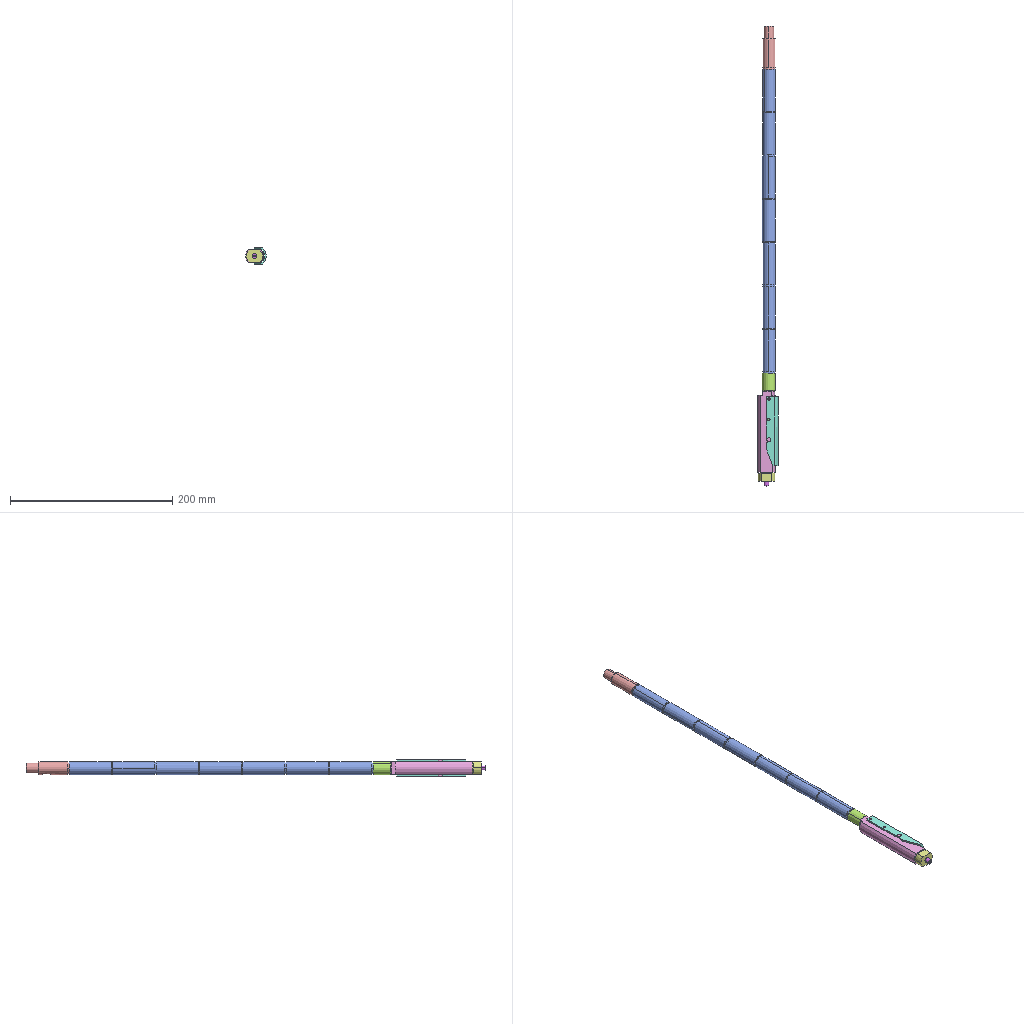Assembly | SolidWorks | 12 different items | 20 placed | box 25 x 567 x 20 mm
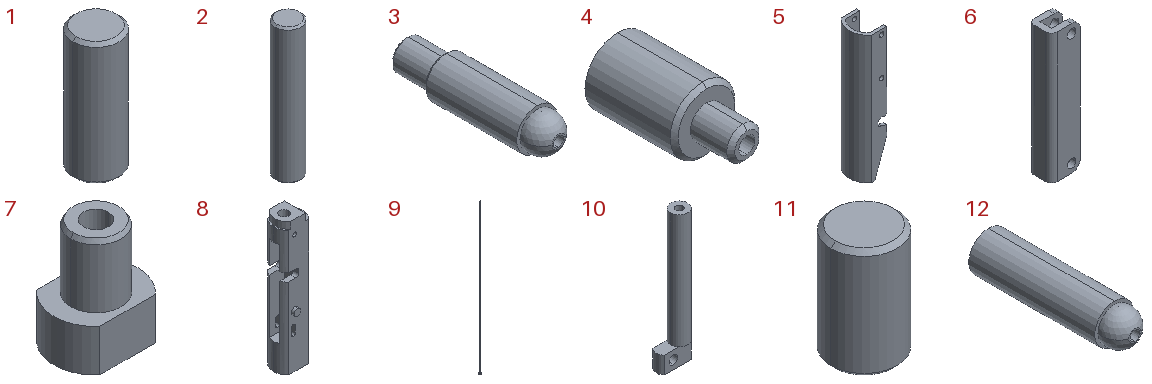Parts list (item | quantity | size | volume | features):
1 | x2 | 3 x 3 x 8 mm | 56.188 mm3 | features Chamfer 1, Extrusion 1
2 | x1 | 3 x 3 x 16 mm | 112.737 mm3 | features Chamfer 1, Extrusion 1
3 | x1 | 16 x 60 x 16 mm | 8216 mm3 | features ICE 3, Chamfer 1, Revolution 1
4 | x1 | 16 x 32 x 16 mm | 3856 mm3 | features Chamfer 1, Revolution 1
5 | x1 | 15 x 20 x 85 mm | 6317 mm3 | features Fillet 2, ICE 2, Extrusion 1
6 | x1 | 10 x 8 x 45 mm | 2011 mm3 | features Extrusion 1, Fillet 1, ICE 1
7 | x1 | 20 x 15 x 25 mm | 3667 mm3 | features ICE 2, Chamfer 1, Extrusion 1
8 | x1 | 22 x 20.4 x 100 mm | 22225 mm3 | features ICE 11, 3DProfileFeature 2, HoleWzd 2, Extrusion 1, MirrorPattern 1
9 | x1 | 6 x 6 x 493 mm | 1623 mm3 | features Chamfer 1, Extrusion 1, ICE 1
10 | x1 | 11 x 6 x 46 mm | 1129 mm3 | features ICE 3, Extrusion 1
11 | x2 | 3 x 3 x 5 mm | 34.983 mm3 | features Chamfer 1, Extrusion 1
12 | x7 | 16 x 60 x 16 mm | 9983 mm3 | features Revolution 1
Mates (type | each side: item.copy, entity, surface, feature):
Concentric | 3.1 face sphere Revolve2 | 12.1 face sphere Revolve2
Concentric | 12.2 face sphere Revolve2 | 12.3 face sphere Revolve2
Concentric | 12.4 face sphere Revolve2 | 12.3 face sphere Revolve2
Concentric | 12.1 face sphere Revolve2 | 12.2 face sphere Revolve2
Concentric | 4.1 face cylinder Revolve2 | 8.1 face cylinder M8 Tapped Hole1
Coincident | 4.1 face plane Revolve2 | 8.1 face plane Boss-Extrude1
Parallel | 3.1 face plane Revolve2 | 12.1 face plane Revolve2
Parallel | 12.1 face plane Revolve2 | 12.2 face plane Revolve2
Parallel | 12.2 face plane Revolve2 | 12.3 face plane Revolve2
Parallel | 12.4 face plane Revolve2 | 12.3 face plane Revolve2
Parallel | 12.4 face plane Revolve2 | 4.1 face plane Revolve2
Concentric | 8.1 face cylinder Mirror3 | 5.1 face cylinder Cut-Extrude1
Coincident | 8.1 face plane Cut-Extrude1 | 5.1 face plane Boss-Extrude1
Parallel | 8.1 face plane Cut-Extrude1 | assembly plane
Coincident | 8.1 face plane Cut-Extrude3 | 6.1 face plane Boss-Extrude1
Slot | 6.1 face cylinder Cut-Extrude1 | 8.1 face plane Cut-Extrude6
Concentric | 5.1 face cylinder Cut-Extrude1 | 6.1 face cylinder Cut-Extrude1
Concentric | 6.1 face cylinder Cut-Extrude1 | 2.1 face cylinder Boss-Extrude1
Coincident | 8.1 face plane Cut-Extrude1 | 2.1 face plane Boss-Extrude1
Concentric | 5.1 face cylinder Cut-Extrude1 | 1.1 face cylinder Boss-Extrude1
Coincident | 5.1 face plane Boss-Extrude1 | 1.1 face plane Boss-Extrude1
Concentric | 5.1 face cylinder Cut-Extrude1 | 1.2 face cylinder Boss-Extrude1
Coincident | 5.1 face plane Boss-Extrude1 | 1.2 face plane Boss-Extrude1
Concentric | 3.1 face cylinder Revolve2 | 9.1 face cylinder Boss-Extrude2
Coincident | 3.1 face plane Revolve2 | 9.1 face plane Boss-Extrude2
Concentric | 8.1 face cylinder Cut-Extrude5 | 11.1 face cylinder Boss-Extrude1
Coincident | 5.1 face plane Boss-Extrude1 | 11.1 face plane Boss-Extrude1
Concentric | 5.1 face cylinder Cut-Extrude1 | 11.2 face cylinder Boss-Extrude1
Coincident | 5.1 face plane Boss-Extrude1 | 11.2 face plane Boss-Extrude1
Concentric | 12.4 face sphere Revolve2 | 12.5 face sphere Revolve2
Parallel | 12.4 face plane Revolve2 | 12.5 face plane Revolve2
Concentric | 12.5 face sphere Revolve2 | 12.6 face sphere Revolve2
Parallel | 12.5 face plane Revolve2 | 12.6 face plane Revolve2
Concentric | 12.6 face sphere Revolve2 | 12.7 face sphere Revolve2
Parallel | 12.6 face plane Revolve2 | 12.7 face plane Revolve2
Concentric | 4.1 face sphere Revolve2 | 12.7 face sphere Revolve2
Parallel | 4.1 face plane Revolve2 | 12.7 face plane Revolve2
Concentric | 8.1 face cylinder M12x1.5 Tapped Hole1 | 7.1 face cylinder Boss-Extrude1
DistanceDim | 8.1 face plane Boss-Extrude1 | 7.1 face plane Boss-Extrude2
Concentric | 7.1 face cylinder Boss-Extrude1 | 10.1 face cylinder Boss-Extrude1
Concentric | 2.1 face cylinder Boss-Extrude1 | 10.1 face cylinder Cut-Extrude2